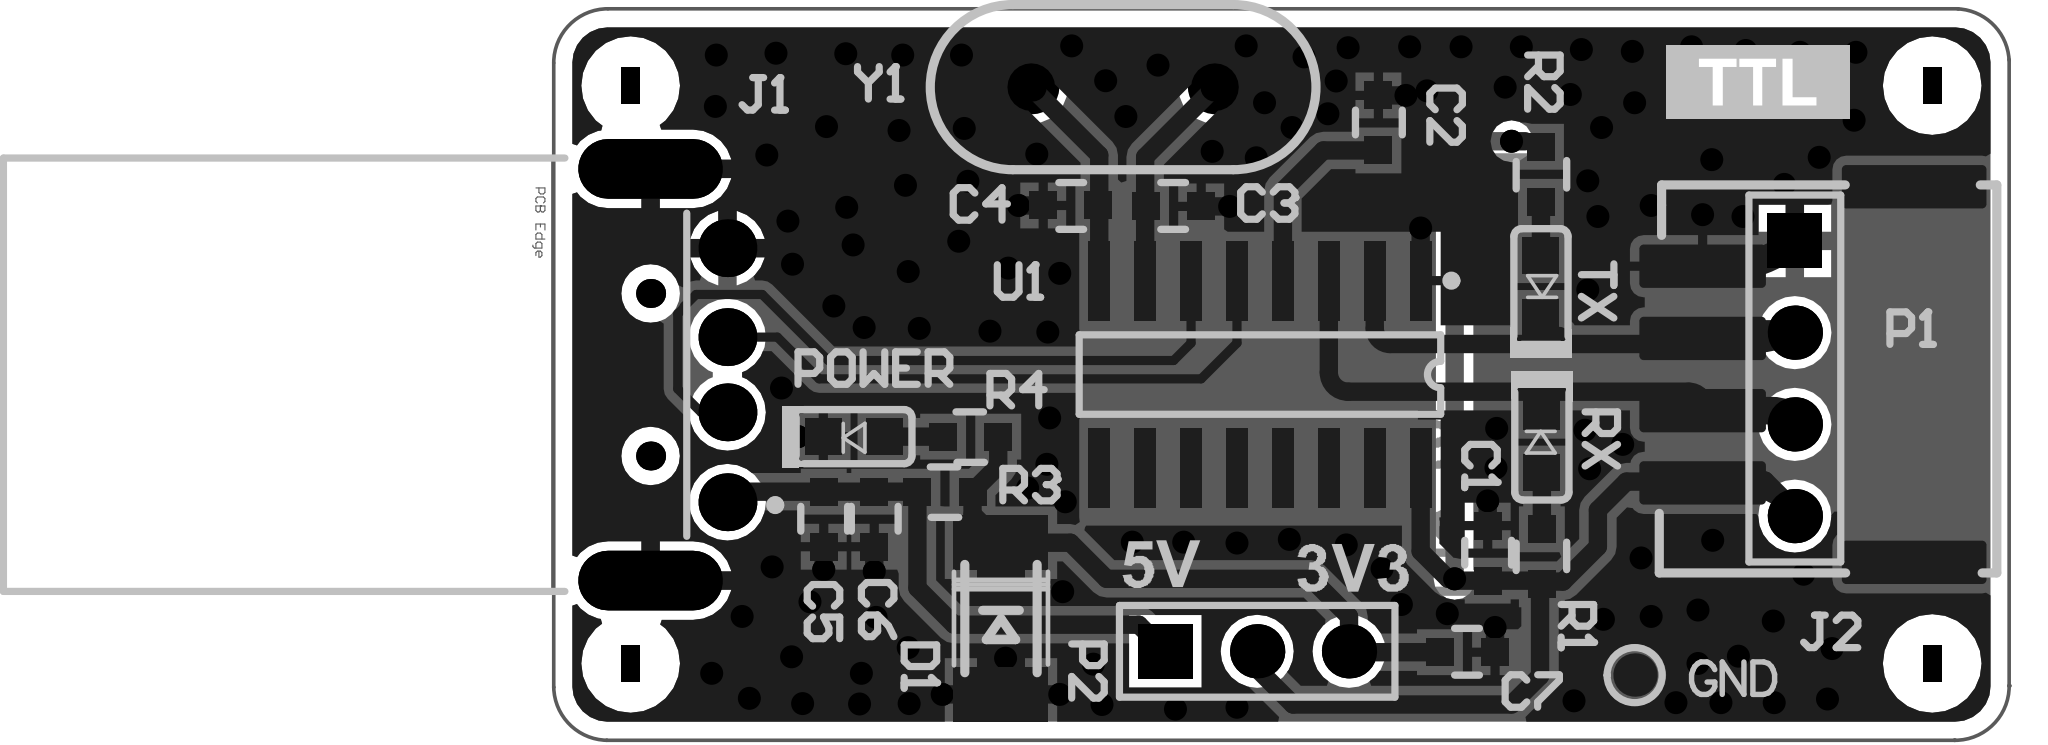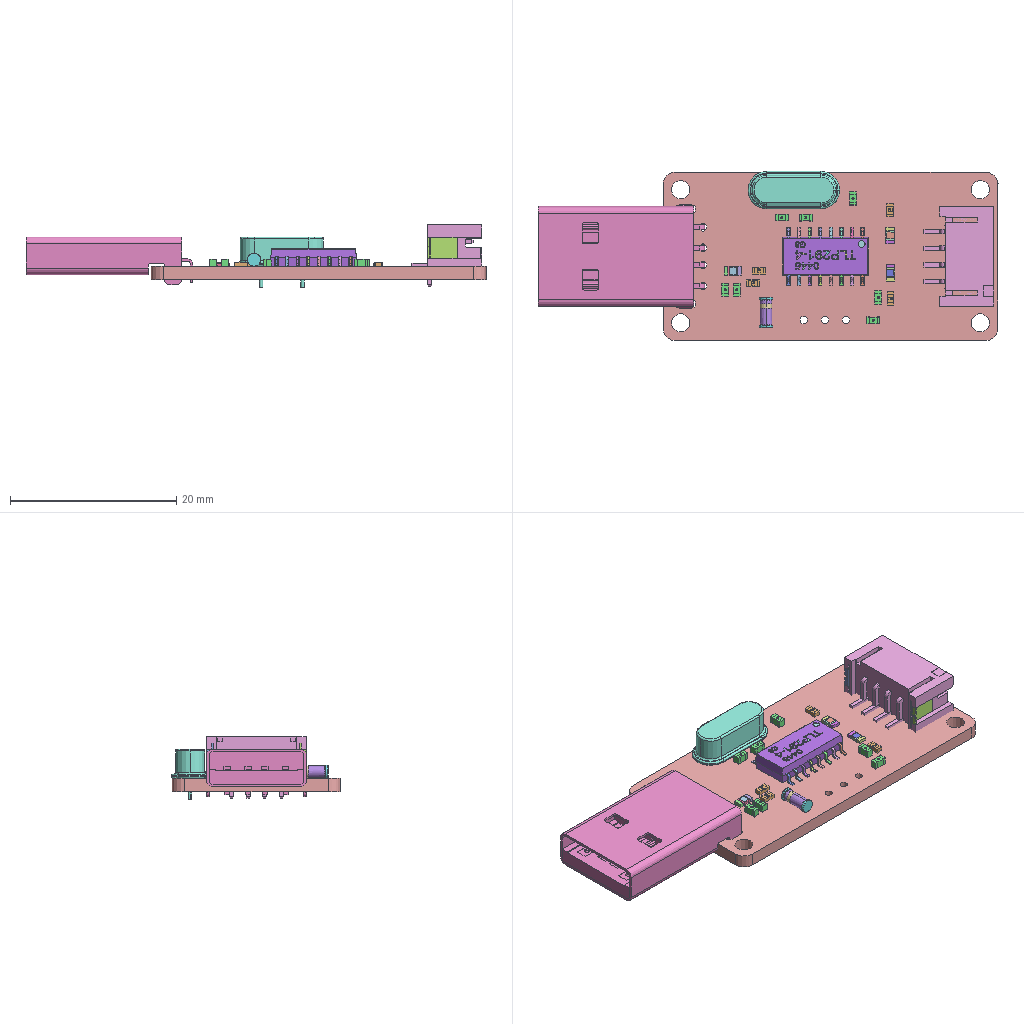Circuit board layout | Altium Designer | box 55.3 x 20.3 x 7.5 mm
Part placement:
Designator,Comment,Layer,Footprint,Center-X(mm),Center-Y(mm),Rotation
GND,Comment,TopLayer,TP_T,29.78,1.68,180
J2,PH2.0/2.54/1.25-SMT-4P,TopLayer,PH2.0-4P-WT,34.575,10,270
Y1,12MHz,TopLayer,XTAL-5.08,15.621,17.958,270
U1,CH340G,TopLayer,SOP16M,19.405,10,180
R4,R,TopLayer,RES0603,11.405,8.28,360
R3,220R,TopLayer,RES0603,10.693,6.756,360
R2,R,TopLayer,RES0603,27.178,15.545,90
R1,R,TopLayer,RES0603,27.203,4.953,270
P2,Header 3,TopLayer,HDR1X3,19.329,2.337,360
P1,Header 4,TopLayer,HDR1X4,34.2,9.89,270
POWER,LED,TopLayer,LED-0603_RED,8.179,8.28,360
TX,LED,TopLayer,LED-0603_RED,27.178,12.437,90
RX,LED,TopLayer,LED-0603_RED,27.203,8.128,270
J1,USB-F-HOLE,TopLayer,USB-F-HOLE,3.615,9.995,270
D1,ZM4733A_C129202,TopLayer,LL-41,12.243,3.243,90
C7,0.1uF,TopLayer,CAP0603,25.146,2.311,180
C6,0.1uF,TopLayer,CAP0603,8.738,5.994,90
C5,0.1uF,TopLayer,CAP0603,7.341,5.994,90
C4,22pF,TopLayer,CAP0603,14.173,14.681,0
C3,22pF,TopLayer,CAP0603,17.018,14.656,180
C2,0.1uF,TopLayer,CAP0603,22.682,16.967,90
C1,0.1uF,TopLayer,CAP0603,25.705,5.055,90